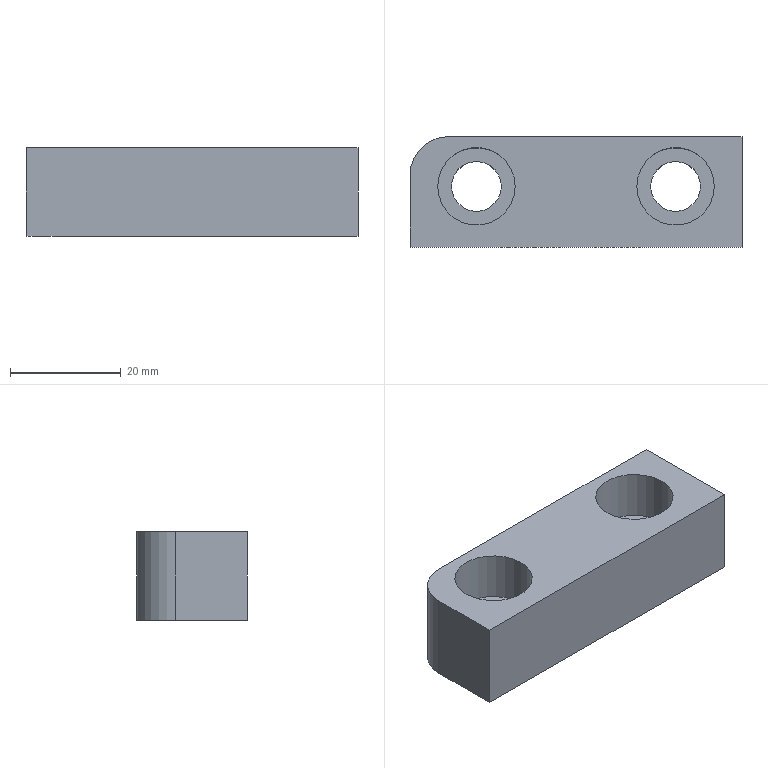Part | STEP file | solid 7 | 1 solid | 13 faces | box 60 x 20 x 16 mm | volume 15370 mm3 | plane 8 | cylinder 5 | commonest cylinder face diameters 14 x3 9 x2